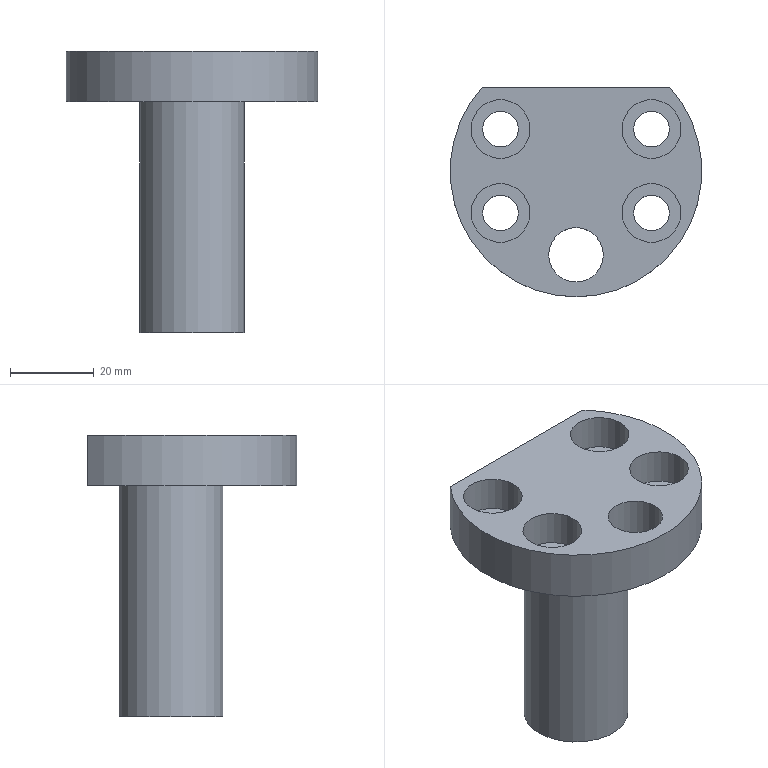Part | NX | 1 solid | 19 faces | box 60 x 50 x 67 mm | volume 49159 mm3 | cylinder 11 | plane 8 | commonest cylinder face diameters 8.5 x4 14 x4 13 x1 24.8 x1 60 x1
STEP:
#1=CARTESIAN_POINT('',(22.25,-10.,-12.));
#2=VERTEX_POINT('',#1);
#3=CARTESIAN_POINT('',(18.,-10.,-12.));
#4=DIRECTION('',(0.,0.,1.));
#5=DIRECTION('',(1.,0.,0.));
#6=AXIS2_PLACEMENT_3D('',#3,#4,#5);
#7=CIRCLE('',#6,4.25);
#8=EDGE_CURVE('',#2,#2,#7,.T.);
#9=ORIENTED_EDGE('',*,*,#8,.F.);
#10=EDGE_LOOP('',(#9));
#11=FACE_BOUND('',#10,.T.);
#12=CARTESIAN_POINT('',(22.25,-10.,-8.5));
#13=VERTEX_POINT('',#12);
#14=CARTESIAN_POINT('',(18.,-10.,-8.5));
#15=DIRECTION('',(0.,0.,1.));
#16=DIRECTION('',(1.,0.,0.));
#17=AXIS2_PLACEMENT_3D('',#14,#15,#16);
#18=CIRCLE('',#17,4.25);
#19=EDGE_CURVE('',#13,#13,#18,.F.);
#20=ORIENTED_EDGE('',*,*,#19,.F.);
#21=EDGE_LOOP('',(#20));
#22=FACE_BOUND('',#21,.T.);
#23=CARTESIAN_POINT('',(18.,-10.,-12.));
#24=DIRECTION('',(0.,0.,1.));
#25=DIRECTION('',(1.,0.,0.));
#26=AXIS2_PLACEMENT_3D('',#23,#24,#25);
#27=CYLINDRICAL_SURFACE('',#26,4.25);
#28=ADVANCED_FACE('',(#11,#22),#27,.F.);
#29=CARTESIAN_POINT('',(-13.75,10.,-12.));
#30=VERTEX_POINT('',#29);
#31=CARTESIAN_POINT('',(-18.,10.,-12.));
#32=DIRECTION('',(0.,0.,1.));
#33=DIRECTION('',(1.,0.,0.));
#34=AXIS2_PLACEMENT_3D('',#31,#32,#33);
#35=CIRCLE('',#34,4.25);
#36=EDGE_CURVE('',#30,#30,#35,.T.);
#37=ORIENTED_EDGE('',*,*,#36,.F.);
#38=EDGE_LOOP('',(#37));
#39=FACE_BOUND('',#38,.T.);
#40=CARTESIAN_POINT('',(-13.75,10.,-8.5));
#41=VERTEX_POINT('',#40);
#42=CARTESIAN_POINT('',(-18.,10.,-8.5));
#43=DIRECTION('',(0.,0.,1.));
#44=DIRECTION('',(1.,0.,0.));
#45=AXIS2_PLACEMENT_3D('',#42,#43,#44);
#46=CIRCLE('',#45,4.25);
#47=EDGE_CURVE('',#41,#41,#46,.F.);
#48=ORIENTED_EDGE('',*,*,#47,.F.);
#49=EDGE_LOOP('',(#48));
#50=FACE_BOUND('',#49,.T.);
#51=CARTESIAN_POINT('',(-18.,10.,-12.));
#52=DIRECTION('',(0.,0.,1.));
#53=DIRECTION('',(1.,0.,0.));
#54=AXIS2_PLACEMENT_3D('',#51,#52,#53);
#55=CYLINDRICAL_SURFACE('',#54,4.25);
#56=ADVANCED_FACE('',(#39,#50),#55,.F.);
#57=CARTESIAN_POINT('',(-13.75,-10.,-12.));
#58=VERTEX_POINT('',#57);
#59=CARTESIAN_POINT('',(-18.,-10.,-12.));
#60=DIRECTION('',(0.,0.,1.));
#61=DIRECTION('',(1.,0.,0.));
#62=AXIS2_PLACEMENT_3D('',#59,#60,#61);
#63=CIRCLE('',#62,4.25);
#64=EDGE_CURVE('',#58,#58,#63,.T.);
#65=ORIENTED_EDGE('',*,*,#64,.F.);
#66=EDGE_LOOP('',(#65));
#67=FACE_BOUND('',#66,.T.);
#68=CARTESIAN_POINT('',(-13.75,-10.,-8.5));
#69=VERTEX_POINT('',#68);
#70=CARTESIAN_POINT('',(-18.,-10.,-8.5));
#71=DIRECTION('',(0.,0.,1.));
#72=DIRECTION('',(1.,0.,0.));
#73=AXIS2_PLACEMENT_3D('',#70,#71,#72);
#74=CIRCLE('',#73,4.25);
#75=EDGE_CURVE('',#69,#69,#74,.F.);
#76=ORIENTED_EDGE('',*,*,#75,.F.);
#77=EDGE_LOOP('',(#76));
#78=FACE_BOUND('',#77,.T.);
#79=CARTESIAN_POINT('',(-18.,-10.,-12.));
#80=DIRECTION('',(0.,0.,1.));
#81=DIRECTION('',(1.,0.,0.));
#82=AXIS2_PLACEMENT_3D('',#79,#80,#81);
#83=CYLINDRICAL_SURFACE('',#82,4.25);
#84=ADVANCED_FACE('',(#67,#78),#83,.F.);
#85=CARTESIAN_POINT('',(22.25,10.,-12.));
#86=VERTEX_POINT('',#85);
#87=CARTESIAN_POINT('',(18.,10.,-12.));
#88=DIRECTION('',(0.,0.,1.));
#89=DIRECTION('',(1.,0.,0.));
#90=AXIS2_PLACEMENT_3D('',#87,#88,#89);
#91=CIRCLE('',#90,4.25);
#92=EDGE_CURVE('',#86,#86,#91,.T.);
#93=ORIENTED_EDGE('',*,*,#92,.F.);
#94=EDGE_LOOP('',(#93));
#95=FACE_BOUND('',#94,.T.);
#96=CARTESIAN_POINT('',(22.25,10.,-8.5));
#97=VERTEX_POINT('',#96);
#98=CARTESIAN_POINT('',(18.,10.,-8.5));
#99=DIRECTION('',(0.,0.,1.));
#100=DIRECTION('',(1.,0.,0.));
#101=AXIS2_PLACEMENT_3D('',#98,#99,#100);
#102=CIRCLE('',#101,4.25);
#103=EDGE_CURVE('',#97,#97,#102,.F.);
#104=ORIENTED_EDGE('',*,*,#103,.F.);
#105=EDGE_LOOP('',(#104));
#106=FACE_BOUND('',#105,.T.);
#107=CARTESIAN_POINT('',(18.,10.,-12.));
#108=DIRECTION('',(0.,0.,1.));
#109=DIRECTION('',(1.,0.,0.));
#110=AXIS2_PLACEMENT_3D('',#107,#108,#109);
#111=CYLINDRICAL_SURFACE('',#110,4.25);
#112=ADVANCED_FACE('',(#95,#106),#111,.F.);
#113=CARTESIAN_POINT('',(-22.361,20.,0.));
#114=VERTEX_POINT('',#113);
#115=CARTESIAN_POINT('',(22.361,20.,0.));
#116=VERTEX_POINT('',#115);
#117=CARTESIAN_POINT('',(0.,0.,0.));
#118=DIRECTION('',(0.,0.,1.));
#119=DIRECTION('',(1.,0.,0.));
#120=AXIS2_PLACEMENT_3D('',#117,#118,#119);
#121=CIRCLE('',#120,30.);
#122=EDGE_CURVE('',#114,#116,#121,.T.);
#123=ORIENTED_EDGE('',*,*,#122,.F.);
#124=CARTESIAN_POINT('',(-22.361,20.,-12.));
#125=VERTEX_POINT('',#124);
#126=CARTESIAN_POINT('',(-22.361,20.,-12.));
#127=DIRECTION('',(0.,0.,1.));
#128=VECTOR('',#127,1000.);
#129=LINE('',#126,#128);
#130=EDGE_CURVE('',#114,#125,#129,.F.);
#131=ORIENTED_EDGE('',*,*,#130,.T.);
#132=CARTESIAN_POINT('',(22.361,20.,-12.));
#133=VERTEX_POINT('',#132);
#134=CARTESIAN_POINT('',(0.,0.,-12.));
#135=DIRECTION('',(0.,0.,1.));
#136=DIRECTION('',(1.,0.,0.));
#137=AXIS2_PLACEMENT_3D('',#134,#135,#136);
#138=CIRCLE('',#137,30.);
#139=EDGE_CURVE('',#125,#133,#138,.T.);
#140=ORIENTED_EDGE('',*,*,#139,.T.);
#141=CARTESIAN_POINT('',(22.361,20.,-12.));
#142=DIRECTION('',(0.,0.,1.));
#143=VECTOR('',#142,1000.);
#144=LINE('',#141,#143);
#145=EDGE_CURVE('',#133,#116,#144,.T.);
#146=ORIENTED_EDGE('',*,*,#145,.T.);
#147=EDGE_LOOP('',(#123,#131,#140,#146));
#148=FACE_BOUND('',#147,.T.);
#149=CARTESIAN_POINT('',(0.,0.,-12.));
#150=DIRECTION('',(0.,0.,1.));
#151=DIRECTION('',(1.,0.,0.));
#152=AXIS2_PLACEMENT_3D('',#149,#150,#151);
#153=CYLINDRICAL_SURFACE('',#152,30.);
#154=ADVANCED_FACE('',(#148),#153,.T.);
#155=CARTESIAN_POINT('',(6.5,-20.,-12.));
#156=VERTEX_POINT('',#155);
#157=CARTESIAN_POINT('',(0.,-20.,-12.));
#158=DIRECTION('',(0.,0.,1.));
#159=DIRECTION('',(1.,0.,0.));
#160=AXIS2_PLACEMENT_3D('',#157,#158,#159);
#161=CIRCLE('',#160,6.5);
#162=EDGE_CURVE('',#156,#156,#161,.T.);
#163=ORIENTED_EDGE('',*,*,#162,.F.);
#164=EDGE_LOOP('',(#163));
#165=FACE_BOUND('',#164,.T.);
#166=CARTESIAN_POINT('',(6.5,-20.,0.));
#167=VERTEX_POINT('',#166);
#168=CARTESIAN_POINT('',(0.,-20.,0.));
#169=DIRECTION('',(0.,0.,1.));
#170=DIRECTION('',(1.,0.,0.));
#171=AXIS2_PLACEMENT_3D('',#168,#169,#170);
#172=CIRCLE('',#171,6.5);
#173=EDGE_CURVE('',#167,#167,#172,.T.);
#174=ORIENTED_EDGE('',*,*,#173,.T.);
#175=EDGE_LOOP('',(#174));
#176=FACE_BOUND('',#175,.T.);
#177=CARTESIAN_POINT('',(0.,-20.,-12.));
#178=DIRECTION('',(0.,0.,1.));
#179=DIRECTION('',(1.,0.,0.));
#180=AXIS2_PLACEMENT_3D('',#177,#178,#179);
#181=CYLINDRICAL_SURFACE('',#180,6.5);
#182=ADVANCED_FACE('',(#165,#176),#181,.F.);
#183=CARTESIAN_POINT('',(22.361,20.,0.));
#184=DIRECTION('',(-1.,0.,0.));
#185=VECTOR('',#184,1000.);
#186=LINE('',#183,#185);
#187=EDGE_CURVE('',#116,#114,#186,.T.);
#188=ORIENTED_EDGE('',*,*,#187,.F.);
#189=ORIENTED_EDGE('',*,*,#145,.F.);
#190=CARTESIAN_POINT('',(22.361,20.,-12.));
#191=DIRECTION('',(-1.,0.,0.));
#192=VECTOR('',#191,1000.);
#193=LINE('',#190,#192);
#194=EDGE_CURVE('',#133,#125,#193,.T.);
#195=ORIENTED_EDGE('',*,*,#194,.T.);
#196=ORIENTED_EDGE('',*,*,#130,.F.);
#197=EDGE_LOOP('',(#188,#189,#195,#196));
#198=FACE_BOUND('',#197,.T.);
#199=CARTESIAN_POINT('',(22.361,20.,-12.));
#200=DIRECTION('',(0.,1.,0.));
#201=DIRECTION('',(0.,0.,1.));
#202=AXIS2_PLACEMENT_3D('',#199,#200,#201);
#203=PLANE('',#202);
#204=ADVANCED_FACE('',(#198),#203,.T.);
#205=ORIENTED_EDGE('',*,*,#139,.F.);
#206=ORIENTED_EDGE('',*,*,#194,.F.);
#207=EDGE_LOOP('',(#205,#206));
#208=FACE_BOUND('',#207,.T.);
#209=ORIENTED_EDGE('',*,*,#64,.T.);
#210=EDGE_LOOP('',(#209));
#211=FACE_BOUND('',#210,.T.);
#212=ORIENTED_EDGE('',*,*,#36,.T.);
#213=EDGE_LOOP('',(#212));
#214=FACE_BOUND('',#213,.T.);
#215=CARTESIAN_POINT('',(12.4,0.,-12.));
#216=VERTEX_POINT('',#215);
#217=CARTESIAN_POINT('',(0.,0.,-12.));
#218=DIRECTION('',(0.,0.,1.));
#219=DIRECTION('',(1.,0.,0.));
#220=AXIS2_PLACEMENT_3D('',#217,#218,#219);
#221=CIRCLE('',#220,12.4);
#222=EDGE_CURVE('',#216,#216,#221,.T.);
#223=ORIENTED_EDGE('',*,*,#222,.T.);
#224=EDGE_LOOP('',(#223));
#225=FACE_BOUND('',#224,.T.);
#226=ORIENTED_EDGE('',*,*,#162,.T.);
#227=EDGE_LOOP('',(#226));
#228=FACE_BOUND('',#227,.T.);
#229=ORIENTED_EDGE('',*,*,#8,.T.);
#230=EDGE_LOOP('',(#229));
#231=FACE_BOUND('',#230,.T.);
#232=ORIENTED_EDGE('',*,*,#92,.T.);
#233=EDGE_LOOP('',(#232));
#234=FACE_BOUND('',#233,.T.);
#235=CARTESIAN_POINT('',(0.,0.,-12.));
#236=DIRECTION('',(0.,0.,1.));
#237=DIRECTION('',(1.,0.,0.));
#238=AXIS2_PLACEMENT_3D('',#235,#236,#237);
#239=PLANE('',#238);
#240=ADVANCED_FACE('',(#208,#211,#214,#225,#228,#231,#234),#239,.F.);
#241=CARTESIAN_POINT('',(25.,-10.,0.));
#242=VERTEX_POINT('',#241);
#243=CARTESIAN_POINT('',(18.,-10.,0.));
#244=DIRECTION('',(0.,0.,1.));
#245=DIRECTION('',(1.,0.,0.));
#246=AXIS2_PLACEMENT_3D('',#243,#244,#245);
#247=CIRCLE('',#246,7.);
#248=EDGE_CURVE('',#242,#242,#247,.T.);
#249=ORIENTED_EDGE('',*,*,#248,.F.);
#250=EDGE_LOOP('',(#249));
#251=FACE_BOUND('',#250,.T.);
#252=CARTESIAN_POINT('',(-11.,10.,0.));
#253=VERTEX_POINT('',#252);
#254=CARTESIAN_POINT('',(-18.,10.,0.));
#255=DIRECTION('',(0.,0.,1.));
#256=DIRECTION('',(1.,0.,0.));
#257=AXIS2_PLACEMENT_3D('',#254,#255,#256);
#258=CIRCLE('',#257,7.);
#259=EDGE_CURVE('',#253,#253,#258,.T.);
#260=ORIENTED_EDGE('',*,*,#259,.F.);
#261=EDGE_LOOP('',(#260));
#262=FACE_BOUND('',#261,.T.);
#263=CARTESIAN_POINT('',(-11.,-10.,0.));
#264=VERTEX_POINT('',#263);
#265=CARTESIAN_POINT('',(-18.,-10.,0.));
#266=DIRECTION('',(0.,0.,1.));
#267=DIRECTION('',(1.,0.,0.));
#268=AXIS2_PLACEMENT_3D('',#265,#266,#267);
#269=CIRCLE('',#268,7.);
#270=EDGE_CURVE('',#264,#264,#269,.T.);
#271=ORIENTED_EDGE('',*,*,#270,.F.);
#272=EDGE_LOOP('',(#271));
#273=FACE_BOUND('',#272,.T.);
#274=CARTESIAN_POINT('',(25.,10.,0.));
#275=VERTEX_POINT('',#274);
#276=CARTESIAN_POINT('',(18.,10.,0.));
#277=DIRECTION('',(0.,0.,1.));
#278=DIRECTION('',(1.,0.,0.));
#279=AXIS2_PLACEMENT_3D('',#276,#277,#278);
#280=CIRCLE('',#279,7.);
#281=EDGE_CURVE('',#275,#275,#280,.T.);
#282=ORIENTED_EDGE('',*,*,#281,.F.);
#283=EDGE_LOOP('',(#282));
#284=FACE_BOUND('',#283,.T.);
#285=ORIENTED_EDGE('',*,*,#122,.T.);
#286=ORIENTED_EDGE('',*,*,#187,.T.);
#287=EDGE_LOOP('',(#285,#286));
#288=FACE_BOUND('',#287,.T.);
#289=ORIENTED_EDGE('',*,*,#173,.F.);
#290=EDGE_LOOP('',(#289));
#291=FACE_BOUND('',#290,.T.);
#292=CARTESIAN_POINT('',(0.,0.,0.));
#293=DIRECTION('',(0.,0.,1.));
#294=DIRECTION('',(1.,0.,0.));
#295=AXIS2_PLACEMENT_3D('',#292,#293,#294);
#296=PLANE('',#295);
#297=ADVANCED_FACE('',(#251,#262,#273,#284,#288,#291),#296,.T.);
#298=CARTESIAN_POINT('',(25.,10.,-8.5));
#299=VERTEX_POINT('',#298);
#300=CARTESIAN_POINT('',(18.,10.,-8.5));
#301=DIRECTION('',(0.,0.,1.));
#302=DIRECTION('',(1.,0.,0.));
#303=AXIS2_PLACEMENT_3D('',#300,#301,#302);
#304=CIRCLE('',#303,7.);
#305=EDGE_CURVE('',#299,#299,#304,.F.);
#306=ORIENTED_EDGE('',*,*,#305,.F.);
#307=EDGE_LOOP('',(#306));
#308=FACE_BOUND('',#307,.T.);
#309=ORIENTED_EDGE('',*,*,#103,.T.);
#310=EDGE_LOOP('',(#309));
#311=FACE_BOUND('',#310,.T.);
#312=CARTESIAN_POINT('',(18.,10.,-8.5));
#313=DIRECTION('',(0.,0.,1.));
#314=DIRECTION('',(1.,0.,0.));
#315=AXIS2_PLACEMENT_3D('',#312,#313,#314);
#316=PLANE('',#315);
#317=ADVANCED_FACE('',(#308,#311),#316,.T.);
#318=ORIENTED_EDGE('',*,*,#305,.T.);
#319=EDGE_LOOP('',(#318));
#320=FACE_BOUND('',#319,.T.);
#321=ORIENTED_EDGE('',*,*,#281,.T.);
#322=EDGE_LOOP('',(#321));
#323=FACE_BOUND('',#322,.T.);
#324=CARTESIAN_POINT('',(18.,10.,-8.5));
#325=DIRECTION('',(0.,0.,1.));
#326=DIRECTION('',(1.,0.,0.));
#327=AXIS2_PLACEMENT_3D('',#324,#325,#326);
#328=CYLINDRICAL_SURFACE('',#327,7.);
#329=ADVANCED_FACE('',(#320,#323),#328,.F.);
#330=CARTESIAN_POINT('',(-11.,-10.,-8.5));
#331=VERTEX_POINT('',#330);
#332=CARTESIAN_POINT('',(-18.,-10.,-8.5));
#333=DIRECTION('',(0.,0.,1.));
#334=DIRECTION('',(1.,0.,0.));
#335=AXIS2_PLACEMENT_3D('',#332,#333,#334);
#336=CIRCLE('',#335,7.);
#337=EDGE_CURVE('',#331,#331,#336,.F.);
#338=ORIENTED_EDGE('',*,*,#337,.F.);
#339=EDGE_LOOP('',(#338));
#340=FACE_BOUND('',#339,.T.);
#341=ORIENTED_EDGE('',*,*,#75,.T.);
#342=EDGE_LOOP('',(#341));
#343=FACE_BOUND('',#342,.T.);
#344=CARTESIAN_POINT('',(-18.,-10.,-8.5));
#345=DIRECTION('',(0.,0.,1.));
#346=DIRECTION('',(1.,0.,0.));
#347=AXIS2_PLACEMENT_3D('',#344,#345,#346);
#348=PLANE('',#347);
#349=ADVANCED_FACE('',(#340,#343),#348,.T.);
#350=ORIENTED_EDGE('',*,*,#337,.T.);
#351=EDGE_LOOP('',(#350));
#352=FACE_BOUND('',#351,.T.);
#353=ORIENTED_EDGE('',*,*,#270,.T.);
#354=EDGE_LOOP('',(#353));
#355=FACE_BOUND('',#354,.T.);
#356=CARTESIAN_POINT('',(-18.,-10.,-8.5));
#357=DIRECTION('',(0.,0.,1.));
#358=DIRECTION('',(1.,0.,0.));
#359=AXIS2_PLACEMENT_3D('',#356,#357,#358);
#360=CYLINDRICAL_SURFACE('',#359,7.);
#361=ADVANCED_FACE('',(#352,#355),#360,.F.);
#362=CARTESIAN_POINT('',(-11.,10.,-8.5));
#363=VERTEX_POINT('',#362);
#364=CARTESIAN_POINT('',(-18.,10.,-8.5));
#365=DIRECTION('',(0.,0.,1.));
#366=DIRECTION('',(1.,0.,0.));
#367=AXIS2_PLACEMENT_3D('',#364,#365,#366);
#368=CIRCLE('',#367,7.);
#369=EDGE_CURVE('',#363,#363,#368,.F.);
#370=ORIENTED_EDGE('',*,*,#369,.F.);
#371=EDGE_LOOP('',(#370));
#372=FACE_BOUND('',#371,.T.);
#373=ORIENTED_EDGE('',*,*,#47,.T.);
#374=EDGE_LOOP('',(#373));
#375=FACE_BOUND('',#374,.T.);
#376=CARTESIAN_POINT('',(-18.,10.,-8.5));
#377=DIRECTION('',(0.,0.,1.));
#378=DIRECTION('',(1.,0.,0.));
#379=AXIS2_PLACEMENT_3D('',#376,#377,#378);
#380=PLANE('',#379);
#381=ADVANCED_FACE('',(#372,#375),#380,.T.);
#382=ORIENTED_EDGE('',*,*,#369,.T.);
#383=EDGE_LOOP('',(#382));
#384=FACE_BOUND('',#383,.T.);
#385=ORIENTED_EDGE('',*,*,#259,.T.);
#386=EDGE_LOOP('',(#385));
#387=FACE_BOUND('',#386,.T.);
#388=CARTESIAN_POINT('',(-18.,10.,-8.5));
#389=DIRECTION('',(0.,0.,1.));
#390=DIRECTION('',(1.,0.,0.));
#391=AXIS2_PLACEMENT_3D('',#388,#389,#390);
#392=CYLINDRICAL_SURFACE('',#391,7.);
#393=ADVANCED_FACE('',(#384,#387),#392,.F.);
#394=CARTESIAN_POINT('',(25.,-10.,-8.5));
#395=VERTEX_POINT('',#394);
#396=CARTESIAN_POINT('',(18.,-10.,-8.5));
#397=DIRECTION('',(0.,0.,1.));
#398=DIRECTION('',(1.,0.,0.));
#399=AXIS2_PLACEMENT_3D('',#396,#397,#398);
#400=CIRCLE('',#399,7.);
#401=EDGE_CURVE('',#395,#395,#400,.F.);
#402=ORIENTED_EDGE('',*,*,#401,.F.);
#403=EDGE_LOOP('',(#402));
#404=FACE_BOUND('',#403,.T.);
#405=ORIENTED_EDGE('',*,*,#19,.T.);
#406=EDGE_LOOP('',(#405));
#407=FACE_BOUND('',#406,.T.);
#408=CARTESIAN_POINT('',(18.,-10.,-8.5));
#409=DIRECTION('',(0.,0.,1.));
#410=DIRECTION('',(1.,0.,0.));
#411=AXIS2_PLACEMENT_3D('',#408,#409,#410);
#412=PLANE('',#411);
#413=ADVANCED_FACE('',(#404,#407),#412,.T.);
#414=ORIENTED_EDGE('',*,*,#401,.T.);
#415=EDGE_LOOP('',(#414));
#416=FACE_BOUND('',#415,.T.);
#417=ORIENTED_EDGE('',*,*,#248,.T.);
#418=EDGE_LOOP('',(#417));
#419=FACE_BOUND('',#418,.T.);
#420=CARTESIAN_POINT('',(18.,-10.,-8.5));
#421=DIRECTION('',(0.,0.,1.));
#422=DIRECTION('',(1.,0.,0.));
#423=AXIS2_PLACEMENT_3D('',#420,#421,#422);
#424=CYLINDRICAL_SURFACE('',#423,7.);
#425=ADVANCED_FACE('',(#416,#419),#424,.F.);
#426=CARTESIAN_POINT('',(12.4,0.,-67.));
#427=VERTEX_POINT('',#426);
#428=CARTESIAN_POINT('',(0.,0.,-67.));
#429=DIRECTION('',(0.,0.,1.));
#430=DIRECTION('',(1.,0.,0.));
#431=AXIS2_PLACEMENT_3D('',#428,#429,#430);
#432=CIRCLE('',#431,12.4);
#433=EDGE_CURVE('',#427,#427,#432,.T.);
#434=ORIENTED_EDGE('',*,*,#433,.T.);
#435=EDGE_LOOP('',(#434));
#436=FACE_BOUND('',#435,.T.);
#437=ORIENTED_EDGE('',*,*,#222,.F.);
#438=EDGE_LOOP('',(#437));
#439=FACE_BOUND('',#438,.T.);
#440=CARTESIAN_POINT('',(0.,0.,-67.));
#441=DIRECTION('',(0.,0.,1.));
#442=DIRECTION('',(1.,0.,0.));
#443=AXIS2_PLACEMENT_3D('',#440,#441,#442);
#444=CYLINDRICAL_SURFACE('',#443,12.4);
#445=ADVANCED_FACE('',(#436,#439),#444,.T.);
#446=ORIENTED_EDGE('',*,*,#433,.F.);
#447=EDGE_LOOP('',(#446));
#448=FACE_BOUND('',#447,.T.);
#449=CARTESIAN_POINT('',(0.,0.,-67.));
#450=DIRECTION('',(0.,0.,1.));
#451=DIRECTION('',(1.,0.,0.));
#452=AXIS2_PLACEMENT_3D('',#449,#450,#451);
#453=PLANE('',#452);
#454=ADVANCED_FACE('',(#448),#453,.F.);
#455=CLOSED_SHELL('',(#28,#56,#84,#112,#154,#182,#204,#240,#297,#317,#329,#349,#361,#381,#393,#413,#425,#445,#454));
#456=MANIFOLD_SOLID_BREP('',#455);
#457=(LENGTH_UNIT()NAMED_UNIT(*)SI_UNIT(.MILLI.,.METRE.));
#458=UNCERTAINTY_MEASURE_WITH_UNIT(LENGTH_MEASURE(0.00001),#457,'','');
#459=(NAMED_UNIT(*)PLANE_ANGLE_UNIT()SI_UNIT($,.RADIAN.));
#460=(NAMED_UNIT(*)SI_UNIT($,.STERADIAN.)SOLID_ANGLE_UNIT());
#461=(GEOMETRIC_REPRESENTATION_CONTEXT(3)GLOBAL_UNCERTAINTY_ASSIGNED_CONTEXT((#458))GLOBAL_UNIT_ASSIGNED_CONTEXT((#457,#459,#460))REPRESENTATION_CONTEXT('',''));
#462=ADVANCED_BREP_SHAPE_REPRESENTATION('',(#456),#461);